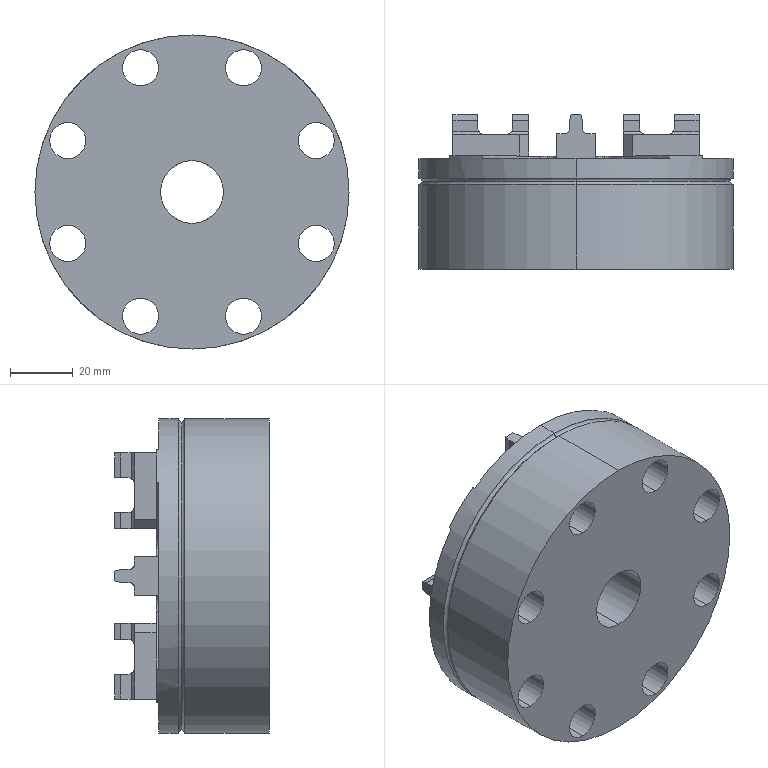Part | SolidWorks | features ICE 7, CirPattern 4, RevCut 3, Chamfer 1, Extrusion 1, Fillet 1, MirrorPattern 1 | 1 solid | 152 faces | box 100 x 49.3 x 100 mm | volume 247149 mm3 | plane 106 | cylinder 40 | torus 4 | sphere 2 | commonest cylinder face diameters 11.5 x16 6 x10 4 x8 100 x4 20 x2